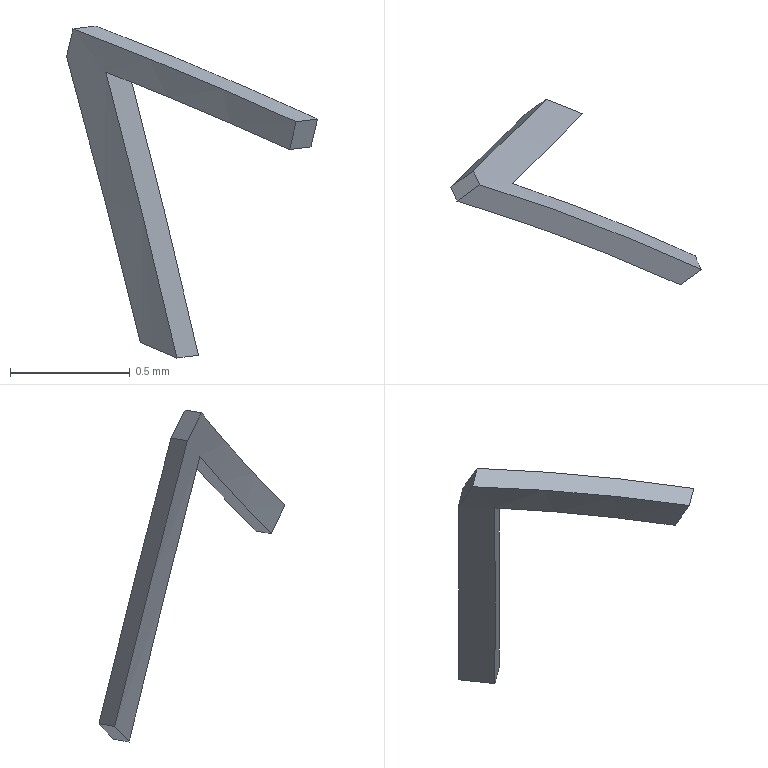Part | SolidWorks | features BaseBody 1 | 1 solid | 9 faces | box 1.048 x 0.7769 x 1.387 mm | volume 0.03423 mm3 | plane 7 | cylinder 2 | commonest cylinder face diameters 16.8 x1 17 x1
STEP:
#1=CARTESIAN_POINT('',(1969.901,-236.399,995.718));
#2=VERTEX_POINT('',#1);
#3=CARTESIAN_POINT('',(1970.198,-236.103,994.523));
#4=VERTEX_POINT('',#3);
#5=CARTESIAN_POINT('',(1969.901,-236.399,995.718));
#6=CARTESIAN_POINT('',(1970.006,-236.296,995.322));
#7=CARTESIAN_POINT('',(1970.105,-236.198,994.924));
#8=CARTESIAN_POINT('',(1970.198,-236.103,994.523));
#9=B_SPLINE_CURVE_WITH_KNOTS('',3,(#5,#6,#7,#8),.UNSPECIFIED.,.F.,.F.,(4,4),(0.,1.),.UNSPECIFIED.);
#10=EDGE_CURVE('',#2,#4,#9,.T.);
#11=ORIENTED_EDGE('',*,*,#10,.F.);
#12=CARTESIAN_POINT('',(1970.669,-236.696,995.393));
#13=VERTEX_POINT('',#12);
#14=CARTESIAN_POINT('',(1966.472,-243.55,992.95));
#15=DIRECTION('',(0.2015,-0.436,0.8771));
#16=DIRECTION('',(-0.7309,-0.6631,-0.1618));
#17=AXIS2_PLACEMENT_3D('',#14,#15,#16);
#18=CIRCLE('',#17,8.4);
#19=EDGE_CURVE('',#13,#2,#18,.T.);
#20=ORIENTED_EDGE('',*,*,#19,.F.);
#21=CARTESIAN_POINT('',(1970.696,-236.754,995.51));
#22=VERTEX_POINT('',#21);
#23=CARTESIAN_POINT('',(1971.647,-238.812,999.65));
#24=DIRECTION('',(0.2015,-0.436,0.8771));
#25=VECTOR('',#24,1000.);
#26=LINE('',#23,#25);
#27=EDGE_CURVE('',#13,#22,#26,.T.);
#28=ORIENTED_EDGE('',*,*,#27,.T.);
#29=CARTESIAN_POINT('',(1969.764,-236.405,995.898));
#30=VERTEX_POINT('',#29);
#31=CARTESIAN_POINT('',(1966.499,-243.608,993.067));
#32=DIRECTION('',(0.2015,-0.436,0.8771));
#33=DIRECTION('',(-0.7309,-0.6631,-0.1618));
#34=AXIS2_PLACEMENT_3D('',#31,#32,#33);
#35=CIRCLE('',#34,8.4);
#36=EDGE_CURVE('',#22,#30,#35,.T.);
#37=ORIENTED_EDGE('',*,*,#36,.T.);
#38=CARTESIAN_POINT('',(1969.737,-236.347,995.781));
#39=VERTEX_POINT('',#38);
#40=CARTESIAN_POINT('',(1970.715,-238.463,1000.038));
#41=DIRECTION('',(-0.2015,0.436,-0.8771));
#42=VECTOR('',#41,1000.);
#43=LINE('',#40,#42);
#44=EDGE_CURVE('',#30,#39,#43,.T.);
#45=ORIENTED_EDGE('',*,*,#44,.T.);
#46=CARTESIAN_POINT('',(1970.045,-236.043,994.588));
#47=VERTEX_POINT('',#46);
#48=CARTESIAN_POINT('',(1969.737,-236.347,995.781));
#49=CARTESIAN_POINT('',(1969.846,-236.241,995.386));
#50=CARTESIAN_POINT('',(1969.949,-236.14,994.988));
#51=CARTESIAN_POINT('',(1970.045,-236.043,994.588));
#52=B_SPLINE_CURVE_WITH_KNOTS('',3,(#48,#49,#50,#51),.UNSPECIFIED.,.F.,.F.,(4,4),(0.,1.),.UNSPECIFIED.);
#53=EDGE_CURVE('',#39,#47,#52,.T.);
#54=ORIENTED_EDGE('',*,*,#53,.T.);
#55=CARTESIAN_POINT('',(1966.247,-243.063,991.97));
#56=DIRECTION('',(-0.2015,0.436,-0.8771));
#57=DIRECTION('',(-0.7309,-0.6631,-0.1618));
#58=AXIS2_PLACEMENT_3D('',#55,#56,#57);
#59=CIRCLE('',#58,8.4);
#60=EDGE_CURVE('',#47,#4,#59,.T.);
#61=ORIENTED_EDGE('',*,*,#60,.T.);
#62=EDGE_LOOP('',(#11,#20,#28,#37,#45,#54,#61));
#63=FACE_OUTER_BOUND('',#62,.T.);
#64=CARTESIAN_POINT('',(1967.45,-245.666,997.207));
#65=DIRECTION('',(0.2015,-0.436,0.8771));
#66=DIRECTION('',(-0.7309,-0.6631,-0.1618));
#67=AXIS2_PLACEMENT_3D('',#64,#65,#66);
#68=CYLINDRICAL_SURFACE('',#67,8.4);
#69=ADVANCED_FACE('',(#63),#68,.F.);
#70=CARTESIAN_POINT('',(1970.288,-236.038,994.534));
#71=VERTEX_POINT('',#70);
#72=CARTESIAN_POINT('',(1970.243,-236.071,994.529));
#73=DIRECTION('',(-0.8088,-0.5792,-0.1022));
#74=VECTOR('',#73,1000.);
#75=LINE('',#72,#74);
#76=EDGE_CURVE('',#71,#4,#75,.T.);
#77=ORIENTED_EDGE('',*,*,#76,.T.);
#78=ORIENTED_EDGE('',*,*,#60,.F.);
#79=CARTESIAN_POINT('',(1970.137,-235.977,994.6));
#80=VERTEX_POINT('',#79);
#81=CARTESIAN_POINT('',(1970.091,-236.01,994.594));
#82=DIRECTION('',(-0.8088,-0.5792,-0.1022));
#83=VECTOR('',#82,1000.);
#84=LINE('',#81,#83);
#85=EDGE_CURVE('',#80,#47,#84,.T.);
#86=ORIENTED_EDGE('',*,*,#85,.F.);
#87=CARTESIAN_POINT('',(1966.247,-243.063,991.97));
#88=DIRECTION('',(-0.2015,0.436,-0.8771));
#89=DIRECTION('',(-0.7309,-0.6631,-0.1618));
#90=AXIS2_PLACEMENT_3D('',#87,#88,#89);
#91=CIRCLE('',#90,8.5);
#92=EDGE_CURVE('',#80,#71,#91,.T.);
#93=ORIENTED_EDGE('',*,*,#92,.T.);
#94=EDGE_LOOP('',(#77,#78,#86,#93));
#95=FACE_OUTER_BOUND('',#94,.T.);
#96=CARTESIAN_POINT('',(1981.656,-238.46,990.719));
#97=DIRECTION('',(-0.2015,0.436,-0.8771));
#98=DIRECTION('',(-0.5526,0.6888,0.4693));
#99=AXIS2_PLACEMENT_3D('',#96,#97,#98);
#100=PLANE('',#99);
#101=ADVANCED_FACE('',(#95),#100,.T.);
#102=ORIENTED_EDGE('',*,*,#85,.T.);
#103=ORIENTED_EDGE('',*,*,#53,.F.);
#104=CARTESIAN_POINT('',(1969.833,-236.279,995.793));
#105=VERTEX_POINT('',#104);
#106=CARTESIAN_POINT('',(1969.785,-236.313,995.787));
#107=DIRECTION('',(-0.8088,-0.5792,-0.1022));
#108=VECTOR('',#107,1000.);
#109=LINE('',#106,#108);
#110=EDGE_CURVE('',#105,#39,#109,.T.);
#111=ORIENTED_EDGE('',*,*,#110,.F.);
#112=CARTESIAN_POINT('',(1969.833,-236.279,995.793));
#113=CARTESIAN_POINT('',(1969.897,-236.216,995.556));
#114=CARTESIAN_POINT('',(1969.96,-236.154,995.318));
#115=CARTESIAN_POINT('',(1970.021,-236.094,995.079));
#116=CARTESIAN_POINT('',(1970.08,-236.035,994.84));
#117=CARTESIAN_POINT('',(1970.137,-235.977,994.6));
#118=B_SPLINE_CURVE_WITH_KNOTS('',5,(#112,#113,#114,#115,#116,#117),.UNSPECIFIED.,.F.,.F.,(6,6),(0.,1.),.UNSPECIFIED.);
#119=EDGE_CURVE('',#105,#80,#118,.T.);
#120=ORIENTED_EDGE('',*,*,#119,.T.);
#121=EDGE_LOOP('',(#102,#103,#111,#120));
#122=FACE_OUTER_BOUND('',#121,.T.);
#123=CARTESIAN_POINT('',(1976.125,-231.772,996.588));
#124=DIRECTION('',(-0.5859,0.8085,0.05472));
#125=DIRECTION('',(-0.05092,-0.1041,0.9933));
#126=AXIS2_PLACEMENT_3D('',#123,#124,#125);
#127=PLANE('',#126);
#128=ADVANCED_FACE('',(#122),#127,.T.);
#129=ORIENTED_EDGE('',*,*,#110,.T.);
#130=ORIENTED_EDGE('',*,*,#44,.F.);
#131=CARTESIAN_POINT('',(1969.859,-236.337,995.91));
#132=VERTEX_POINT('',#131);
#133=CARTESIAN_POINT('',(1969.812,-236.371,995.904));
#134=DIRECTION('',(-0.8088,-0.5792,-0.1022));
#135=VECTOR('',#134,1000.);
#136=LINE('',#133,#135);
#137=EDGE_CURVE('',#132,#30,#136,.T.);
#138=ORIENTED_EDGE('',*,*,#137,.F.);
#139=CARTESIAN_POINT('',(1969.846,-236.308,995.851));
#140=DIRECTION('',(-0.2015,0.436,-0.8771));
#141=VECTOR('',#140,1000.);
#142=LINE('',#139,#141);
#143=EDGE_CURVE('',#132,#105,#142,.T.);
#144=ORIENTED_EDGE('',*,*,#143,.T.);
#145=EDGE_LOOP('',(#129,#130,#138,#144));
#146=FACE_OUTER_BOUND('',#145,.T.);
#147=CARTESIAN_POINT('',(1976.152,-231.83,996.705));
#148=DIRECTION('',(-0.5526,0.6888,0.4693));
#149=DIRECTION('',(0.2015,-0.436,0.8771));
#150=AXIS2_PLACEMENT_3D('',#147,#148,#149);
#151=PLANE('',#150);
#152=ADVANCED_FACE('',(#146),#151,.T.);
#153=ORIENTED_EDGE('',*,*,#137,.T.);
#154=ORIENTED_EDGE('',*,*,#36,.F.);
#155=CARTESIAN_POINT('',(1970.785,-236.69,995.521));
#156=VERTEX_POINT('',#155);
#157=CARTESIAN_POINT('',(1970.74,-236.722,995.516));
#158=DIRECTION('',(-0.8088,-0.5792,-0.1022));
#159=VECTOR('',#158,1000.);
#160=LINE('',#157,#159);
#161=EDGE_CURVE('',#156,#22,#160,.T.);
#162=ORIENTED_EDGE('',*,*,#161,.F.);
#163=CARTESIAN_POINT('',(1966.499,-243.608,993.067));
#164=DIRECTION('',(0.2015,-0.436,0.8771));
#165=DIRECTION('',(-0.7309,-0.6631,-0.1618));
#166=AXIS2_PLACEMENT_3D('',#163,#164,#165);
#167=CIRCLE('',#166,8.5);
#168=EDGE_CURVE('',#156,#132,#167,.T.);
#169=ORIENTED_EDGE('',*,*,#168,.T.);
#170=EDGE_LOOP('',(#153,#154,#162,#169));
#171=FACE_OUTER_BOUND('',#170,.T.);
#172=CARTESIAN_POINT('',(1982.253,-239.435,991.522));
#173=DIRECTION('',(0.2015,-0.436,0.8771));
#174=DIRECTION('',(0.5526,-0.6888,-0.4693));
#175=AXIS2_PLACEMENT_3D('',#172,#173,#174);
#176=PLANE('',#175);
#177=ADVANCED_FACE('',(#171),#176,.T.);
#178=ORIENTED_EDGE('',*,*,#161,.T.);
#179=ORIENTED_EDGE('',*,*,#27,.F.);
#180=CARTESIAN_POINT('',(1970.758,-236.632,995.405));
#181=VERTEX_POINT('',#180);
#182=CARTESIAN_POINT('',(1970.714,-236.664,995.399));
#183=DIRECTION('',(-0.8088,-0.5792,-0.1022));
#184=VECTOR('',#183,1000.);
#185=LINE('',#182,#184);
#186=EDGE_CURVE('',#181,#13,#185,.T.);
#187=ORIENTED_EDGE('',*,*,#186,.F.);
#188=CARTESIAN_POINT('',(1970.772,-236.661,995.463));
#189=DIRECTION('',(0.2015,-0.436,0.8771));
#190=VECTOR('',#189,1000.);
#191=LINE('',#188,#190);
#192=EDGE_CURVE('',#181,#156,#191,.T.);
#193=ORIENTED_EDGE('',*,*,#192,.T.);
#194=EDGE_LOOP('',(#178,#179,#187,#193));
#195=FACE_OUTER_BOUND('',#194,.T.);
#196=CARTESIAN_POINT('',(1976.643,-232.418,996.148));
#197=DIRECTION('',(0.5526,-0.6888,-0.4693));
#198=DIRECTION('',(-0.2015,0.436,-0.8771));
#199=AXIS2_PLACEMENT_3D('',#196,#197,#198);
#200=PLANE('',#199);
#201=ADVANCED_FACE('',(#195),#200,.T.);
#202=CARTESIAN_POINT('',(1969.996,-236.331,995.73));
#203=VERTEX_POINT('',#202);
#204=CARTESIAN_POINT('',(1966.472,-243.55,992.95));
#205=DIRECTION('',(0.2015,-0.436,0.8771));
#206=DIRECTION('',(-0.7309,-0.6631,-0.1618));
#207=AXIS2_PLACEMENT_3D('',#204,#205,#206);
#208=CIRCLE('',#207,8.5);
#209=EDGE_CURVE('',#181,#203,#208,.T.);
#210=ORIENTED_EDGE('',*,*,#209,.F.);
#211=ORIENTED_EDGE('',*,*,#186,.T.);
#212=ORIENTED_EDGE('',*,*,#19,.T.);
#213=CARTESIAN_POINT('',(1969.948,-236.365,995.724));
#214=DIRECTION('',(-0.8088,-0.5792,-0.1022));
#215=VECTOR('',#214,1000.);
#216=LINE('',#213,#215);
#217=EDGE_CURVE('',#203,#2,#216,.T.);
#218=ORIENTED_EDGE('',*,*,#217,.F.);
#219=EDGE_LOOP('',(#210,#211,#212,#218));
#220=FACE_OUTER_BOUND('',#219,.T.);
#221=CARTESIAN_POINT('',(1977.06,-232.938,995.794));
#222=DIRECTION('',(0.2015,-0.436,0.8771));
#223=DIRECTION('',(0.5526,-0.6888,-0.4693));
#224=AXIS2_PLACEMENT_3D('',#221,#222,#223);
#225=PLANE('',#224);
#226=ADVANCED_FACE('',(#220),#225,.F.);
#227=ORIENTED_EDGE('',*,*,#217,.T.);
#228=ORIENTED_EDGE('',*,*,#10,.T.);
#229=ORIENTED_EDGE('',*,*,#76,.F.);
#230=CARTESIAN_POINT('',(1969.996,-236.331,995.73));
#231=CARTESIAN_POINT('',(1970.058,-236.27,995.492));
#232=CARTESIAN_POINT('',(1970.118,-236.21,995.254));
#233=CARTESIAN_POINT('',(1970.176,-236.152,995.015));
#234=CARTESIAN_POINT('',(1970.233,-236.094,994.775));
#235=CARTESIAN_POINT('',(1970.288,-236.038,994.534));
#236=B_SPLINE_CURVE_WITH_KNOTS('',5,(#230,#231,#232,#233,#234,#235),.UNSPECIFIED.,.F.,.F.,(6,6),(0.,1.),.UNSPECIFIED.);
#237=EDGE_CURVE('',#203,#71,#236,.T.);
#238=ORIENTED_EDGE('',*,*,#237,.F.);
#239=EDGE_LOOP('',(#227,#228,#229,#238));
#240=FACE_OUTER_BOUND('',#239,.T.);
#241=CARTESIAN_POINT('',(1976.274,-231.752,995.291));
#242=DIRECTION('',(0.5859,-0.8085,-0.05472));
#243=DIRECTION('',(0.05092,0.1041,-0.9933));
#244=AXIS2_PLACEMENT_3D('',#241,#242,#243);
#245=PLANE('',#244);
#246=ADVANCED_FACE('',(#240),#245,.T.);
#247=ORIENTED_EDGE('',*,*,#92,.F.);
#248=ORIENTED_EDGE('',*,*,#119,.F.);
#249=ORIENTED_EDGE('',*,*,#143,.F.);
#250=ORIENTED_EDGE('',*,*,#168,.F.);
#251=ORIENTED_EDGE('',*,*,#192,.F.);
#252=ORIENTED_EDGE('',*,*,#209,.T.);
#253=ORIENTED_EDGE('',*,*,#237,.T.);
#254=EDGE_LOOP('',(#247,#248,#249,#250,#251,#252,#253));
#255=FACE_OUTER_BOUND('',#254,.T.);
#256=CARTESIAN_POINT('',(1967.45,-245.666,997.207));
#257=DIRECTION('',(0.2015,-0.436,0.8771));
#258=DIRECTION('',(-0.7309,-0.6631,-0.1618));
#259=AXIS2_PLACEMENT_3D('',#256,#257,#258);
#260=CYLINDRICAL_SURFACE('',#259,8.5);
#261=ADVANCED_FACE('',(#255),#260,.T.);
#262=CLOSED_SHELL('',(#69,#101,#128,#152,#177,#201,#226,#246,#261));
#263=MANIFOLD_SOLID_BREP('',#262);
#264=CARTESIAN_POINT('',(0.,0.,0.));
#265=DIRECTION('',(0.,0.,1.));
#266=DIRECTION('',(1.,0.,0.));
#267=AXIS2_PLACEMENT_3D('',#264,#265,#266);
#268=(LENGTH_UNIT()NAMED_UNIT(*)SI_UNIT(.MILLI.,.METRE.));
#269=UNCERTAINTY_MEASURE_WITH_UNIT(LENGTH_MEASURE(0.00001),#268,'','');
#270=(NAMED_UNIT(*)PLANE_ANGLE_UNIT()SI_UNIT($,.RADIAN.));
#271=(NAMED_UNIT(*)SI_UNIT($,.STERADIAN.)SOLID_ANGLE_UNIT());
#272=(GEOMETRIC_REPRESENTATION_CONTEXT(3)GLOBAL_UNCERTAINTY_ASSIGNED_CONTEXT((#269))GLOBAL_UNIT_ASSIGNED_CONTEXT((#268,#270,#271))REPRESENTATION_CONTEXT('',''));
#273=ADVANCED_BREP_SHAPE_REPRESENTATION('',(#263,#267),#272);